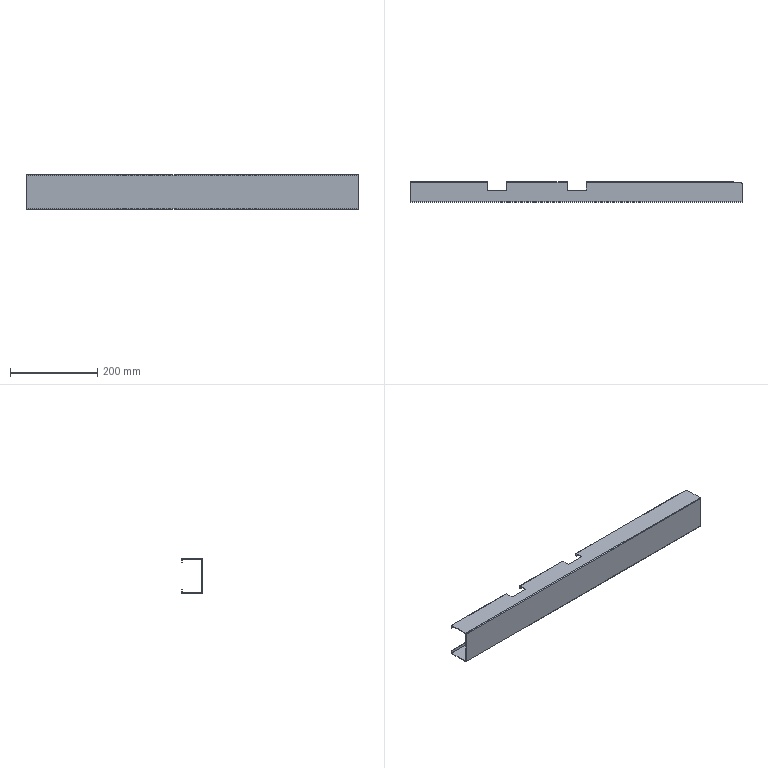Part | 1 solid | 92 faces | box 763 x 48 x 80 mm | volume 203601 mm3 | plane 74 | cylinder 18 | commonest cylinder face diameters 0.4 x8 3.4 x8 6 x2